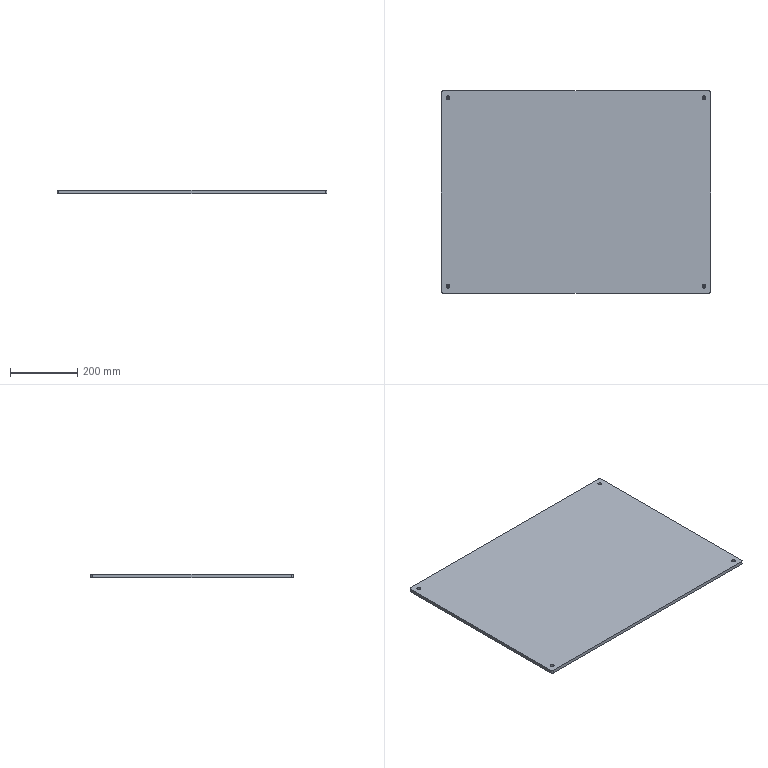Part | SolidWorks | features Extrusion 1, Fillet 1, HoleWzd 1 | 1 solid | 30 faces | box 800 x 600 x 10 mm | volume 4796860 mm3 | cylinder 20 | plane 10 | commonest cylinder face diameters 6.6 x8 11 x8 10 x4
STEP:
#1=CARTESIAN_POINT('',(-385.5,280.,3.6));
#2=VERTEX_POINT('',#1);
#3=CARTESIAN_POINT('',(-374.5,280.,3.6));
#4=VERTEX_POINT('',#3);
#5=CARTESIAN_POINT('',(-380.,280.,3.6));
#6=DIRECTION('',(0.,0.,1.));
#7=DIRECTION('',(1.,0.,0.));
#8=AXIS2_PLACEMENT_3D('',#5,#6,#7);
#9=CIRCLE('',#8,5.5);
#10=EDGE_CURVE('',#2,#4,#9,.T.);
#11=ORIENTED_EDGE('',*,*,#10,.F.);
#12=CARTESIAN_POINT('',(-385.5,280.,10.));
#13=VERTEX_POINT('',#12);
#14=CARTESIAN_POINT('',(-385.5,280.,10.));
#15=DIRECTION('',(0.,0.,1.));
#16=VECTOR('',#15,1000.);
#17=LINE('',#14,#16);
#18=EDGE_CURVE('',#2,#13,#17,.T.);
#19=ORIENTED_EDGE('',*,*,#18,.T.);
#20=CARTESIAN_POINT('',(-374.5,280.,10.));
#21=VERTEX_POINT('',#20);
#22=CARTESIAN_POINT('',(-380.,280.,10.));
#23=DIRECTION('',(0.,0.,1.));
#24=DIRECTION('',(1.,0.,0.));
#25=AXIS2_PLACEMENT_3D('',#22,#23,#24);
#26=CIRCLE('',#25,5.5);
#27=EDGE_CURVE('',#13,#21,#26,.T.);
#28=ORIENTED_EDGE('',*,*,#27,.T.);
#29=CARTESIAN_POINT('',(-374.5,280.,10.));
#30=DIRECTION('',(0.,0.,1.));
#31=VECTOR('',#30,1000.);
#32=LINE('',#29,#31);
#33=EDGE_CURVE('',#4,#21,#32,.T.);
#34=ORIENTED_EDGE('',*,*,#33,.F.);
#35=EDGE_LOOP('',(#11,#19,#28,#34));
#36=FACE_OUTER_BOUND('',#35,.T.);
#37=CARTESIAN_POINT('',(-380.,280.,10.));
#38=DIRECTION('',(0.,0.,1.));
#39=DIRECTION('',(1.,0.,0.));
#40=AXIS2_PLACEMENT_3D('',#37,#38,#39);
#41=CYLINDRICAL_SURFACE('',#40,5.5);
#42=ADVANCED_FACE('',(#36),#41,.F.);
#43=CARTESIAN_POINT('',(-383.3,280.,0.));
#44=VERTEX_POINT('',#43);
#45=CARTESIAN_POINT('',(-376.7,280.,0.));
#46=VERTEX_POINT('',#45);
#47=CARTESIAN_POINT('',(-380.,280.,0.));
#48=DIRECTION('',(0.,0.,1.));
#49=DIRECTION('',(1.,0.,0.));
#50=AXIS2_PLACEMENT_3D('',#47,#48,#49);
#51=CIRCLE('',#50,3.3);
#52=EDGE_CURVE('',#44,#46,#51,.T.);
#53=ORIENTED_EDGE('',*,*,#52,.F.);
#54=CARTESIAN_POINT('',(-383.3,280.,3.6));
#55=VERTEX_POINT('',#54);
#56=CARTESIAN_POINT('',(-383.3,280.,10.));
#57=DIRECTION('',(0.,0.,1.));
#58=VECTOR('',#57,1000.);
#59=LINE('',#56,#58);
#60=EDGE_CURVE('',#44,#55,#59,.T.);
#61=ORIENTED_EDGE('',*,*,#60,.T.);
#62=CARTESIAN_POINT('',(-376.7,280.,3.6));
#63=VERTEX_POINT('',#62);
#64=CARTESIAN_POINT('',(-380.,280.,3.6));
#65=DIRECTION('',(0.,0.,1.));
#66=DIRECTION('',(1.,0.,0.));
#67=AXIS2_PLACEMENT_3D('',#64,#65,#66);
#68=CIRCLE('',#67,3.3);
#69=EDGE_CURVE('',#55,#63,#68,.T.);
#70=ORIENTED_EDGE('',*,*,#69,.T.);
#71=CARTESIAN_POINT('',(-376.7,280.,10.));
#72=DIRECTION('',(0.,0.,1.));
#73=VECTOR('',#72,1000.);
#74=LINE('',#71,#73);
#75=EDGE_CURVE('',#46,#63,#74,.T.);
#76=ORIENTED_EDGE('',*,*,#75,.F.);
#77=EDGE_LOOP('',(#53,#61,#70,#76));
#78=FACE_OUTER_BOUND('',#77,.T.);
#79=CARTESIAN_POINT('',(-380.,280.,10.));
#80=DIRECTION('',(0.,0.,1.));
#81=DIRECTION('',(1.,0.,0.));
#82=AXIS2_PLACEMENT_3D('',#79,#80,#81);
#83=CYLINDRICAL_SURFACE('',#82,3.3);
#84=ADVANCED_FACE('',(#78),#83,.F.);
#85=CARTESIAN_POINT('',(374.5,280.,3.6));
#86=VERTEX_POINT('',#85);
#87=CARTESIAN_POINT('',(385.5,280.,3.6));
#88=VERTEX_POINT('',#87);
#89=CARTESIAN_POINT('',(380.,280.,3.6));
#90=DIRECTION('',(0.,0.,1.));
#91=DIRECTION('',(1.,0.,0.));
#92=AXIS2_PLACEMENT_3D('',#89,#90,#91);
#93=CIRCLE('',#92,5.5);
#94=EDGE_CURVE('',#86,#88,#93,.T.);
#95=ORIENTED_EDGE('',*,*,#94,.F.);
#96=CARTESIAN_POINT('',(374.5,280.,10.));
#97=VERTEX_POINT('',#96);
#98=CARTESIAN_POINT('',(374.5,280.,10.));
#99=DIRECTION('',(0.,0.,1.));
#100=VECTOR('',#99,1000.);
#101=LINE('',#98,#100);
#102=EDGE_CURVE('',#86,#97,#101,.T.);
#103=ORIENTED_EDGE('',*,*,#102,.T.);
#104=CARTESIAN_POINT('',(385.5,280.,10.));
#105=VERTEX_POINT('',#104);
#106=CARTESIAN_POINT('',(380.,280.,10.));
#107=DIRECTION('',(0.,0.,1.));
#108=DIRECTION('',(1.,0.,0.));
#109=AXIS2_PLACEMENT_3D('',#106,#107,#108);
#110=CIRCLE('',#109,5.5);
#111=EDGE_CURVE('',#97,#105,#110,.T.);
#112=ORIENTED_EDGE('',*,*,#111,.T.);
#113=CARTESIAN_POINT('',(385.5,280.,10.));
#114=DIRECTION('',(0.,0.,1.));
#115=VECTOR('',#114,1000.);
#116=LINE('',#113,#115);
#117=EDGE_CURVE('',#88,#105,#116,.T.);
#118=ORIENTED_EDGE('',*,*,#117,.F.);
#119=EDGE_LOOP('',(#95,#103,#112,#118));
#120=FACE_OUTER_BOUND('',#119,.T.);
#121=CARTESIAN_POINT('',(380.,280.,10.));
#122=DIRECTION('',(0.,0.,1.));
#123=DIRECTION('',(1.,0.,0.));
#124=AXIS2_PLACEMENT_3D('',#121,#122,#123);
#125=CYLINDRICAL_SURFACE('',#124,5.5);
#126=ADVANCED_FACE('',(#120),#125,.F.);
#127=CARTESIAN_POINT('',(376.7,280.,0.));
#128=VERTEX_POINT('',#127);
#129=CARTESIAN_POINT('',(383.3,280.,0.));
#130=VERTEX_POINT('',#129);
#131=CARTESIAN_POINT('',(380.,280.,0.));
#132=DIRECTION('',(0.,0.,1.));
#133=DIRECTION('',(1.,0.,0.));
#134=AXIS2_PLACEMENT_3D('',#131,#132,#133);
#135=CIRCLE('',#134,3.3);
#136=EDGE_CURVE('',#128,#130,#135,.T.);
#137=ORIENTED_EDGE('',*,*,#136,.F.);
#138=CARTESIAN_POINT('',(376.7,280.,3.6));
#139=VERTEX_POINT('',#138);
#140=CARTESIAN_POINT('',(376.7,280.,10.));
#141=DIRECTION('',(0.,0.,1.));
#142=VECTOR('',#141,1000.);
#143=LINE('',#140,#142);
#144=EDGE_CURVE('',#128,#139,#143,.T.);
#145=ORIENTED_EDGE('',*,*,#144,.T.);
#146=CARTESIAN_POINT('',(383.3,280.,3.6));
#147=VERTEX_POINT('',#146);
#148=CARTESIAN_POINT('',(380.,280.,3.6));
#149=DIRECTION('',(0.,0.,1.));
#150=DIRECTION('',(1.,0.,0.));
#151=AXIS2_PLACEMENT_3D('',#148,#149,#150);
#152=CIRCLE('',#151,3.3);
#153=EDGE_CURVE('',#139,#147,#152,.T.);
#154=ORIENTED_EDGE('',*,*,#153,.T.);
#155=CARTESIAN_POINT('',(383.3,280.,10.));
#156=DIRECTION('',(0.,0.,1.));
#157=VECTOR('',#156,1000.);
#158=LINE('',#155,#157);
#159=EDGE_CURVE('',#130,#147,#158,.T.);
#160=ORIENTED_EDGE('',*,*,#159,.F.);
#161=EDGE_LOOP('',(#137,#145,#154,#160));
#162=FACE_OUTER_BOUND('',#161,.T.);
#163=CARTESIAN_POINT('',(380.,280.,10.));
#164=DIRECTION('',(0.,0.,1.));
#165=DIRECTION('',(1.,0.,0.));
#166=AXIS2_PLACEMENT_3D('',#163,#164,#165);
#167=CYLINDRICAL_SURFACE('',#166,3.3);
#168=ADVANCED_FACE('',(#162),#167,.F.);
#169=CARTESIAN_POINT('',(374.5,-280.,3.6));
#170=VERTEX_POINT('',#169);
#171=CARTESIAN_POINT('',(385.5,-280.,3.6));
#172=VERTEX_POINT('',#171);
#173=CARTESIAN_POINT('',(380.,-280.,3.6));
#174=DIRECTION('',(0.,0.,1.));
#175=DIRECTION('',(1.,0.,0.));
#176=AXIS2_PLACEMENT_3D('',#173,#174,#175);
#177=CIRCLE('',#176,5.5);
#178=EDGE_CURVE('',#170,#172,#177,.T.);
#179=ORIENTED_EDGE('',*,*,#178,.F.);
#180=CARTESIAN_POINT('',(374.5,-280.,10.));
#181=VERTEX_POINT('',#180);
#182=CARTESIAN_POINT('',(374.5,-280.,10.));
#183=DIRECTION('',(0.,0.,1.));
#184=VECTOR('',#183,1000.);
#185=LINE('',#182,#184);
#186=EDGE_CURVE('',#170,#181,#185,.T.);
#187=ORIENTED_EDGE('',*,*,#186,.T.);
#188=CARTESIAN_POINT('',(385.5,-280.,10.));
#189=VERTEX_POINT('',#188);
#190=CARTESIAN_POINT('',(380.,-280.,10.));
#191=DIRECTION('',(0.,0.,1.));
#192=DIRECTION('',(1.,0.,0.));
#193=AXIS2_PLACEMENT_3D('',#190,#191,#192);
#194=CIRCLE('',#193,5.5);
#195=EDGE_CURVE('',#181,#189,#194,.T.);
#196=ORIENTED_EDGE('',*,*,#195,.T.);
#197=CARTESIAN_POINT('',(385.5,-280.,10.));
#198=DIRECTION('',(0.,0.,1.));
#199=VECTOR('',#198,1000.);
#200=LINE('',#197,#199);
#201=EDGE_CURVE('',#172,#189,#200,.T.);
#202=ORIENTED_EDGE('',*,*,#201,.F.);
#203=EDGE_LOOP('',(#179,#187,#196,#202));
#204=FACE_OUTER_BOUND('',#203,.T.);
#205=CARTESIAN_POINT('',(380.,-280.,10.));
#206=DIRECTION('',(0.,0.,1.));
#207=DIRECTION('',(1.,0.,0.));
#208=AXIS2_PLACEMENT_3D('',#205,#206,#207);
#209=CYLINDRICAL_SURFACE('',#208,5.5);
#210=ADVANCED_FACE('',(#204),#209,.F.);
#211=CARTESIAN_POINT('',(376.7,-280.,0.));
#212=VERTEX_POINT('',#211);
#213=CARTESIAN_POINT('',(383.3,-280.,0.));
#214=VERTEX_POINT('',#213);
#215=CARTESIAN_POINT('',(380.,-280.,0.));
#216=DIRECTION('',(0.,0.,1.));
#217=DIRECTION('',(1.,0.,0.));
#218=AXIS2_PLACEMENT_3D('',#215,#216,#217);
#219=CIRCLE('',#218,3.3);
#220=EDGE_CURVE('',#212,#214,#219,.T.);
#221=ORIENTED_EDGE('',*,*,#220,.F.);
#222=CARTESIAN_POINT('',(376.7,-280.,3.6));
#223=VERTEX_POINT('',#222);
#224=CARTESIAN_POINT('',(376.7,-280.,10.));
#225=DIRECTION('',(0.,0.,1.));
#226=VECTOR('',#225,1000.);
#227=LINE('',#224,#226);
#228=EDGE_CURVE('',#212,#223,#227,.T.);
#229=ORIENTED_EDGE('',*,*,#228,.T.);
#230=CARTESIAN_POINT('',(383.3,-280.,3.6));
#231=VERTEX_POINT('',#230);
#232=CARTESIAN_POINT('',(380.,-280.,3.6));
#233=DIRECTION('',(0.,0.,1.));
#234=DIRECTION('',(1.,0.,0.));
#235=AXIS2_PLACEMENT_3D('',#232,#233,#234);
#236=CIRCLE('',#235,3.3);
#237=EDGE_CURVE('',#223,#231,#236,.T.);
#238=ORIENTED_EDGE('',*,*,#237,.T.);
#239=CARTESIAN_POINT('',(383.3,-280.,10.));
#240=DIRECTION('',(0.,0.,1.));
#241=VECTOR('',#240,1000.);
#242=LINE('',#239,#241);
#243=EDGE_CURVE('',#214,#231,#242,.T.);
#244=ORIENTED_EDGE('',*,*,#243,.F.);
#245=EDGE_LOOP('',(#221,#229,#238,#244));
#246=FACE_OUTER_BOUND('',#245,.T.);
#247=CARTESIAN_POINT('',(380.,-280.,10.));
#248=DIRECTION('',(0.,0.,1.));
#249=DIRECTION('',(1.,0.,0.));
#250=AXIS2_PLACEMENT_3D('',#247,#248,#249);
#251=CYLINDRICAL_SURFACE('',#250,3.3);
#252=ADVANCED_FACE('',(#246),#251,.F.);
#253=CARTESIAN_POINT('',(-385.5,-280.,3.6));
#254=VERTEX_POINT('',#253);
#255=CARTESIAN_POINT('',(-374.5,-280.,3.6));
#256=VERTEX_POINT('',#255);
#257=CARTESIAN_POINT('',(-380.,-280.,3.6));
#258=DIRECTION('',(0.,0.,1.));
#259=DIRECTION('',(1.,0.,0.));
#260=AXIS2_PLACEMENT_3D('',#257,#258,#259);
#261=CIRCLE('',#260,5.5);
#262=EDGE_CURVE('',#254,#256,#261,.T.);
#263=ORIENTED_EDGE('',*,*,#262,.F.);
#264=CARTESIAN_POINT('',(-385.5,-280.,10.));
#265=VERTEX_POINT('',#264);
#266=CARTESIAN_POINT('',(-385.5,-280.,10.));
#267=DIRECTION('',(0.,0.,1.));
#268=VECTOR('',#267,1000.);
#269=LINE('',#266,#268);
#270=EDGE_CURVE('',#254,#265,#269,.T.);
#271=ORIENTED_EDGE('',*,*,#270,.T.);
#272=CARTESIAN_POINT('',(-374.5,-280.,10.));
#273=VERTEX_POINT('',#272);
#274=CARTESIAN_POINT('',(-380.,-280.,10.));
#275=DIRECTION('',(0.,0.,1.));
#276=DIRECTION('',(1.,0.,0.));
#277=AXIS2_PLACEMENT_3D('',#274,#275,#276);
#278=CIRCLE('',#277,5.5);
#279=EDGE_CURVE('',#265,#273,#278,.T.);
#280=ORIENTED_EDGE('',*,*,#279,.T.);
#281=CARTESIAN_POINT('',(-374.5,-280.,10.));
#282=DIRECTION('',(0.,0.,1.));
#283=VECTOR('',#282,1000.);
#284=LINE('',#281,#283);
#285=EDGE_CURVE('',#256,#273,#284,.T.);
#286=ORIENTED_EDGE('',*,*,#285,.F.);
#287=EDGE_LOOP('',(#263,#271,#280,#286));
#288=FACE_OUTER_BOUND('',#287,.T.);
#289=CARTESIAN_POINT('',(-380.,-280.,10.));
#290=DIRECTION('',(0.,0.,1.));
#291=DIRECTION('',(1.,0.,0.));
#292=AXIS2_PLACEMENT_3D('',#289,#290,#291);
#293=CYLINDRICAL_SURFACE('',#292,5.5);
#294=ADVANCED_FACE('',(#288),#293,.F.);
#295=CARTESIAN_POINT('',(-383.3,-280.,0.));
#296=VERTEX_POINT('',#295);
#297=CARTESIAN_POINT('',(-376.7,-280.,0.));
#298=VERTEX_POINT('',#297);
#299=CARTESIAN_POINT('',(-380.,-280.,0.));
#300=DIRECTION('',(0.,0.,1.));
#301=DIRECTION('',(1.,0.,0.));
#302=AXIS2_PLACEMENT_3D('',#299,#300,#301);
#303=CIRCLE('',#302,3.3);
#304=EDGE_CURVE('',#296,#298,#303,.T.);
#305=ORIENTED_EDGE('',*,*,#304,.F.);
#306=CARTESIAN_POINT('',(-383.3,-280.,3.6));
#307=VERTEX_POINT('',#306);
#308=CARTESIAN_POINT('',(-383.3,-280.,10.));
#309=DIRECTION('',(0.,0.,1.));
#310=VECTOR('',#309,1000.);
#311=LINE('',#308,#310);
#312=EDGE_CURVE('',#296,#307,#311,.T.);
#313=ORIENTED_EDGE('',*,*,#312,.T.);
#314=CARTESIAN_POINT('',(-376.7,-280.,3.6));
#315=VERTEX_POINT('',#314);
#316=CARTESIAN_POINT('',(-380.,-280.,3.6));
#317=DIRECTION('',(0.,0.,1.));
#318=DIRECTION('',(1.,0.,0.));
#319=AXIS2_PLACEMENT_3D('',#316,#317,#318);
#320=CIRCLE('',#319,3.3);
#321=EDGE_CURVE('',#307,#315,#320,.T.);
#322=ORIENTED_EDGE('',*,*,#321,.T.);
#323=CARTESIAN_POINT('',(-376.7,-280.,10.));
#324=DIRECTION('',(0.,0.,1.));
#325=VECTOR('',#324,1000.);
#326=LINE('',#323,#325);
#327=EDGE_CURVE('',#298,#315,#326,.T.);
#328=ORIENTED_EDGE('',*,*,#327,.F.);
#329=EDGE_LOOP('',(#305,#313,#322,#328));
#330=FACE_OUTER_BOUND('',#329,.T.);
#331=CARTESIAN_POINT('',(-380.,-280.,10.));
#332=DIRECTION('',(0.,0.,1.));
#333=DIRECTION('',(1.,0.,0.));
#334=AXIS2_PLACEMENT_3D('',#331,#332,#333);
#335=CYLINDRICAL_SURFACE('',#334,3.3);
#336=ADVANCED_FACE('',(#330),#335,.F.);
#337=CARTESIAN_POINT('',(400.,-295.,0.));
#338=VERTEX_POINT('',#337);
#339=CARTESIAN_POINT('',(400.,295.,0.));
#340=VERTEX_POINT('',#339);
#341=CARTESIAN_POINT('',(400.,300.,0.));
#342=DIRECTION('',(0.,1.,0.));
#343=VECTOR('',#342,1000.);
#344=LINE('',#341,#343);
#345=EDGE_CURVE('',#338,#340,#344,.T.);
#346=ORIENTED_EDGE('',*,*,#345,.T.);
#347=CARTESIAN_POINT('',(400.,295.,10.));
#348=VERTEX_POINT('',#347);
#349=CARTESIAN_POINT('',(400.,295.,10.));
#350=DIRECTION('',(0.,0.,1.));
#351=VECTOR('',#350,1000.);
#352=LINE('',#349,#351);
#353=EDGE_CURVE('',#340,#348,#352,.T.);
#354=ORIENTED_EDGE('',*,*,#353,.T.);
#355=CARTESIAN_POINT('',(400.,-295.,10.));
#356=VERTEX_POINT('',#355);
#357=CARTESIAN_POINT('',(400.,300.,10.));
#358=DIRECTION('',(0.,1.,0.));
#359=VECTOR('',#358,1000.);
#360=LINE('',#357,#359);
#361=EDGE_CURVE('',#356,#348,#360,.T.);
#362=ORIENTED_EDGE('',*,*,#361,.F.);
#363=CARTESIAN_POINT('',(400.,-295.,10.));
#364=DIRECTION('',(0.,0.,-1.));
#365=VECTOR('',#364,1000.);
#366=LINE('',#363,#365);
#367=EDGE_CURVE('',#356,#338,#366,.T.);
#368=ORIENTED_EDGE('',*,*,#367,.T.);
#369=EDGE_LOOP('',(#346,#354,#362,#368));
#370=FACE_OUTER_BOUND('',#369,.T.);
#371=CARTESIAN_POINT('',(400.,300.,10.));
#372=DIRECTION('',(-1.,0.,0.));
#373=DIRECTION('',(0.,0.,1.));
#374=AXIS2_PLACEMENT_3D('',#371,#372,#373);
#375=PLANE('',#374);
#376=ADVANCED_FACE('',(#370),#375,.F.);
#377=CARTESIAN_POINT('',(395.,300.,10.));
#378=VERTEX_POINT('',#377);
#379=CARTESIAN_POINT('',(-395.,300.,10.));
#380=VERTEX_POINT('',#379);
#381=CARTESIAN_POINT('',(-400.,300.,10.));
#382=DIRECTION('',(-1.,0.,0.));
#383=VECTOR('',#382,1000.);
#384=LINE('',#381,#383);
#385=EDGE_CURVE('',#378,#380,#384,.T.);
#386=ORIENTED_EDGE('',*,*,#385,.F.);
#387=CARTESIAN_POINT('',(395.,300.,0.));
#388=VERTEX_POINT('',#387);
#389=CARTESIAN_POINT('',(395.,300.,10.));
#390=DIRECTION('',(0.,0.,-1.));
#391=VECTOR('',#390,1000.);
#392=LINE('',#389,#391);
#393=EDGE_CURVE('',#378,#388,#392,.T.);
#394=ORIENTED_EDGE('',*,*,#393,.T.);
#395=CARTESIAN_POINT('',(-395.,300.,0.));
#396=VERTEX_POINT('',#395);
#397=CARTESIAN_POINT('',(-400.,300.,0.));
#398=DIRECTION('',(-1.,0.,0.));
#399=VECTOR('',#398,1000.);
#400=LINE('',#397,#399);
#401=EDGE_CURVE('',#388,#396,#400,.T.);
#402=ORIENTED_EDGE('',*,*,#401,.T.);
#403=CARTESIAN_POINT('',(-395.,300.,10.));
#404=DIRECTION('',(0.,0.,1.));
#405=VECTOR('',#404,1000.);
#406=LINE('',#403,#405);
#407=EDGE_CURVE('',#396,#380,#406,.T.);
#408=ORIENTED_EDGE('',*,*,#407,.T.);
#409=EDGE_LOOP('',(#386,#394,#402,#408));
#410=FACE_OUTER_BOUND('',#409,.T.);
#411=CARTESIAN_POINT('',(-400.,300.,10.));
#412=DIRECTION('',(0.,-1.,0.));
#413=DIRECTION('',(0.,0.,-1.));
#414=AXIS2_PLACEMENT_3D('',#411,#412,#413);
#415=PLANE('',#414);
#416=ADVANCED_FACE('',(#410),#415,.F.);
#417=CARTESIAN_POINT('',(-400.,295.,0.));
#418=VERTEX_POINT('',#417);
#419=CARTESIAN_POINT('',(-400.,-295.,0.));
#420=VERTEX_POINT('',#419);
#421=CARTESIAN_POINT('',(-400.,300.,0.));
#422=DIRECTION('',(0.,-1.,0.));
#423=VECTOR('',#422,1000.);
#424=LINE('',#421,#423);
#425=EDGE_CURVE('',#418,#420,#424,.T.);
#426=ORIENTED_EDGE('',*,*,#425,.T.);
#427=CARTESIAN_POINT('',(-400.,-295.,10.));
#428=VERTEX_POINT('',#427);
#429=CARTESIAN_POINT('',(-400.,-295.,10.));
#430=DIRECTION('',(0.,0.,1.));
#431=VECTOR('',#430,1000.);
#432=LINE('',#429,#431);
#433=EDGE_CURVE('',#420,#428,#432,.T.);
#434=ORIENTED_EDGE('',*,*,#433,.T.);
#435=CARTESIAN_POINT('',(-400.,295.,10.));
#436=VERTEX_POINT('',#435);
#437=CARTESIAN_POINT('',(-400.,300.,10.));
#438=DIRECTION('',(0.,-1.,0.));
#439=VECTOR('',#438,1000.);
#440=LINE('',#437,#439);
#441=EDGE_CURVE('',#436,#428,#440,.T.);
#442=ORIENTED_EDGE('',*,*,#441,.F.);
#443=CARTESIAN_POINT('',(-400.,295.,10.));
#444=DIRECTION('',(0.,0.,-1.));
#445=VECTOR('',#444,1000.);
#446=LINE('',#443,#445);
#447=EDGE_CURVE('',#436,#418,#446,.T.);
#448=ORIENTED_EDGE('',*,*,#447,.T.);
#449=EDGE_LOOP('',(#426,#434,#442,#448));
#450=FACE_OUTER_BOUND('',#449,.T.);
#451=CARTESIAN_POINT('',(-400.,300.,10.));
#452=DIRECTION('',(1.,0.,0.));
#453=DIRECTION('',(0.,0.,-1.));
#454=AXIS2_PLACEMENT_3D('',#451,#452,#453);
#455=PLANE('',#454);
#456=ADVANCED_FACE('',(#450),#455,.F.);
#457=CARTESIAN_POINT('',(-395.,-300.,0.));
#458=VERTEX_POINT('',#457);
#459=CARTESIAN_POINT('',(395.,-300.,0.));
#460=VERTEX_POINT('',#459);
#461=CARTESIAN_POINT('',(-400.,-300.,0.));
#462=DIRECTION('',(1.,0.,0.));
#463=VECTOR('',#462,1000.);
#464=LINE('',#461,#463);
#465=EDGE_CURVE('',#458,#460,#464,.T.);
#466=ORIENTED_EDGE('',*,*,#465,.T.);
#467=CARTESIAN_POINT('',(395.,-300.,10.));
#468=VERTEX_POINT('',#467);
#469=CARTESIAN_POINT('',(395.,-300.,10.));
#470=DIRECTION('',(0.,0.,1.));
#471=VECTOR('',#470,1000.);
#472=LINE('',#469,#471);
#473=EDGE_CURVE('',#460,#468,#472,.T.);
#474=ORIENTED_EDGE('',*,*,#473,.T.);
#475=CARTESIAN_POINT('',(-395.,-300.,10.));
#476=VERTEX_POINT('',#475);
#477=CARTESIAN_POINT('',(-400.,-300.,10.));
#478=DIRECTION('',(1.,0.,0.));
#479=VECTOR('',#478,1000.);
#480=LINE('',#477,#479);
#481=EDGE_CURVE('',#476,#468,#480,.T.);
#482=ORIENTED_EDGE('',*,*,#481,.F.);
#483=CARTESIAN_POINT('',(-395.,-300.,10.));
#484=DIRECTION('',(0.,0.,-1.));
#485=VECTOR('',#484,1000.);
#486=LINE('',#483,#485);
#487=EDGE_CURVE('',#476,#458,#486,.T.);
#488=ORIENTED_EDGE('',*,*,#487,.T.);
#489=EDGE_LOOP('',(#466,#474,#482,#488));
#490=FACE_OUTER_BOUND('',#489,.T.);
#491=CARTESIAN_POINT('',(-400.,-300.,10.));
#492=DIRECTION('',(0.,1.,0.));
#493=DIRECTION('',(0.,0.,1.));
#494=AXIS2_PLACEMENT_3D('',#491,#492,#493);
#495=PLANE('',#494);
#496=ADVANCED_FACE('',(#490),#495,.F.);
#497=CARTESIAN_POINT('',(-380.,280.,10.));
#498=DIRECTION('',(0.,0.,1.));
#499=DIRECTION('',(1.,0.,0.));
#500=AXIS2_PLACEMENT_3D('',#497,#498,#499);
#501=CIRCLE('',#500,5.5);
#502=EDGE_CURVE('',#21,#13,#501,.T.);
#503=ORIENTED_EDGE('',*,*,#502,.F.);
#504=ORIENTED_EDGE('',*,*,#27,.F.);
#505=EDGE_LOOP('',(#503,#504));
#506=FACE_BOUND('',#505,.T.);
#507=CARTESIAN_POINT('',(380.,280.,10.));
#508=DIRECTION('',(0.,0.,1.));
#509=DIRECTION('',(1.,0.,0.));
#510=AXIS2_PLACEMENT_3D('',#507,#508,#509);
#511=CIRCLE('',#510,5.5);
#512=EDGE_CURVE('',#105,#97,#511,.T.);
#513=ORIENTED_EDGE('',*,*,#512,.F.);
#514=ORIENTED_EDGE('',*,*,#111,.F.);
#515=EDGE_LOOP('',(#513,#514));
#516=FACE_BOUND('',#515,.T.);
#517=CARTESIAN_POINT('',(380.,-280.,10.));
#518=DIRECTION('',(0.,0.,1.));
#519=DIRECTION('',(1.,0.,0.));
#520=AXIS2_PLACEMENT_3D('',#517,#518,#519);
#521=CIRCLE('',#520,5.5);
#522=EDGE_CURVE('',#189,#181,#521,.T.);
#523=ORIENTED_EDGE('',*,*,#522,.F.);
#524=ORIENTED_EDGE('',*,*,#195,.F.);
#525=EDGE_LOOP('',(#523,#524));
#526=FACE_BOUND('',#525,.T.);
#527=CARTESIAN_POINT('',(-380.,-280.,10.));
#528=DIRECTION('',(0.,0.,1.));
#529=DIRECTION('',(1.,0.,0.));
#530=AXIS2_PLACEMENT_3D('',#527,#528,#529);
#531=CIRCLE('',#530,5.5);
#532=EDGE_CURVE('',#273,#265,#531,.T.);
#533=ORIENTED_EDGE('',*,*,#532,.F.);
#534=ORIENTED_EDGE('',*,*,#279,.F.);
#535=EDGE_LOOP('',(#533,#534));
#536=FACE_BOUND('',#535,.T.);
#537=ORIENTED_EDGE('',*,*,#361,.T.);
#538=CARTESIAN_POINT('',(395.,295.,10.));
#539=DIRECTION('',(0.,0.,1.));
#540=DIRECTION('',(1.,0.,0.));
#541=AXIS2_PLACEMENT_3D('',#538,#539,#540);
#542=CIRCLE('',#541,5.);
#543=EDGE_CURVE('',#348,#378,#542,.T.);
#544=ORIENTED_EDGE('',*,*,#543,.T.);
#545=ORIENTED_EDGE('',*,*,#385,.T.);
#546=CARTESIAN_POINT('',(-395.,295.,10.));
#547=DIRECTION('',(0.,0.,1.));
#548=DIRECTION('',(1.,0.,0.));
#549=AXIS2_PLACEMENT_3D('',#546,#547,#548);
#550=CIRCLE('',#549,5.);
#551=EDGE_CURVE('',#380,#436,#550,.T.);
#552=ORIENTED_EDGE('',*,*,#551,.T.);
#553=ORIENTED_EDGE('',*,*,#441,.T.);
#554=CARTESIAN_POINT('',(-395.,-295.,10.));
#555=DIRECTION('',(0.,0.,1.));
#556=DIRECTION('',(1.,0.,0.));
#557=AXIS2_PLACEMENT_3D('',#554,#555,#556);
#558=CIRCLE('',#557,5.);
#559=EDGE_CURVE('',#428,#476,#558,.T.);
#560=ORIENTED_EDGE('',*,*,#559,.T.);
#561=ORIENTED_EDGE('',*,*,#481,.T.);
#562=CARTESIAN_POINT('',(395.,-295.,10.));
#563=DIRECTION('',(0.,0.,1.));
#564=DIRECTION('',(1.,0.,0.));
#565=AXIS2_PLACEMENT_3D('',#562,#563,#564);
#566=CIRCLE('',#565,5.);
#567=EDGE_CURVE('',#468,#356,#566,.T.);
#568=ORIENTED_EDGE('',*,*,#567,.T.);
#569=EDGE_LOOP('',(#537,#544,#545,#552,#553,#560,#561,#568));
#570=FACE_OUTER_BOUND('',#569,.T.);
#571=CARTESIAN_POINT('',(0.,0.,10.));
#572=DIRECTION('',(0.,0.,1.));
#573=DIRECTION('',(1.,0.,0.));
#574=AXIS2_PLACEMENT_3D('',#571,#572,#573);
#575=PLANE('',#574);
#576=ADVANCED_FACE('',(#506,#516,#526,#536,#570),#575,.T.);
#577=CARTESIAN_POINT('',(-380.,280.,0.));
#578=DIRECTION('',(0.,0.,1.));
#579=DIRECTION('',(1.,0.,0.));
#580=AXIS2_PLACEMENT_3D('',#577,#578,#579);
#581=CIRCLE('',#580,3.3);
#582=EDGE_CURVE('',#46,#44,#581,.T.);
#583=ORIENTED_EDGE('',*,*,#582,.T.);
#584=ORIENTED_EDGE('',*,*,#52,.T.);
#585=EDGE_LOOP('',(#583,#584));
#586=FACE_BOUND('',#585,.T.);
#587=CARTESIAN_POINT('',(380.,280.,0.));
#588=DIRECTION('',(0.,0.,1.));
#589=DIRECTION('',(1.,0.,0.));
#590=AXIS2_PLACEMENT_3D('',#587,#588,#589);
#591=CIRCLE('',#590,3.3);
#592=EDGE_CURVE('',#130,#128,#591,.T.);
#593=ORIENTED_EDGE('',*,*,#592,.T.);
#594=ORIENTED_EDGE('',*,*,#136,.T.);
#595=EDGE_LOOP('',(#593,#594));
#596=FACE_BOUND('',#595,.T.);
#597=CARTESIAN_POINT('',(380.,-280.,0.));
#598=DIRECTION('',(0.,0.,1.));
#599=DIRECTION('',(1.,0.,0.));
#600=AXIS2_PLACEMENT_3D('',#597,#598,#599);
#601=CIRCLE('',#600,3.3);
#602=EDGE_CURVE('',#214,#212,#601,.T.);
#603=ORIENTED_EDGE('',*,*,#602,.T.);
#604=ORIENTED_EDGE('',*,*,#220,.T.);
#605=EDGE_LOOP('',(#603,#604));
#606=FACE_BOUND('',#605,.T.);
#607=CARTESIAN_POINT('',(-380.,-280.,0.));
#608=DIRECTION('',(0.,0.,1.));
#609=DIRECTION('',(1.,0.,0.));
#610=AXIS2_PLACEMENT_3D('',#607,#608,#609);
#611=CIRCLE('',#610,3.3);
#612=EDGE_CURVE('',#298,#296,#611,.T.);
#613=ORIENTED_EDGE('',*,*,#612,.T.);
#614=ORIENTED_EDGE('',*,*,#304,.T.);
#615=EDGE_LOOP('',(#613,#614));
#616=FACE_BOUND('',#615,.T.);
#617=ORIENTED_EDGE('',*,*,#401,.F.);
#618=CARTESIAN_POINT('',(395.,295.,0.));
#619=DIRECTION('',(0.,0.,-1.));
#620=DIRECTION('',(1.,0.,0.));
#621=AXIS2_PLACEMENT_3D('',#618,#619,#620);
#622=CIRCLE('',#621,5.);
#623=EDGE_CURVE('',#388,#340,#622,.T.);
#624=ORIENTED_EDGE('',*,*,#623,.T.);
#625=ORIENTED_EDGE('',*,*,#345,.F.);
#626=CARTESIAN_POINT('',(395.,-295.,0.));
#627=DIRECTION('',(0.,0.,-1.));
#628=DIRECTION('',(1.,0.,0.));
#629=AXIS2_PLACEMENT_3D('',#626,#627,#628);
#630=CIRCLE('',#629,5.);
#631=EDGE_CURVE('',#338,#460,#630,.T.);
#632=ORIENTED_EDGE('',*,*,#631,.T.);
#633=ORIENTED_EDGE('',*,*,#465,.F.);
#634=CARTESIAN_POINT('',(-395.,-295.,0.));
#635=DIRECTION('',(0.,0.,-1.));
#636=DIRECTION('',(1.,0.,0.));
#637=AXIS2_PLACEMENT_3D('',#634,#635,#636);
#638=CIRCLE('',#637,5.);
#639=EDGE_CURVE('',#458,#420,#638,.T.);
#640=ORIENTED_EDGE('',*,*,#639,.T.);
#641=ORIENTED_EDGE('',*,*,#425,.F.);
#642=CARTESIAN_POINT('',(-395.,295.,0.));
#643=DIRECTION('',(0.,0.,-1.));
#644=DIRECTION('',(1.,0.,0.));
#645=AXIS2_PLACEMENT_3D('',#642,#643,#644);
#646=CIRCLE('',#645,5.);
#647=EDGE_CURVE('',#418,#396,#646,.T.);
#648=ORIENTED_EDGE('',*,*,#647,.T.);
#649=EDGE_LOOP('',(#617,#624,#625,#632,#633,#640,#641,#648));
#650=FACE_OUTER_BOUND('',#649,.T.);
#651=CARTESIAN_POINT('',(0.,0.,0.));
#652=DIRECTION('',(0.,0.,1.));
#653=DIRECTION('',(1.,0.,0.));
#654=AXIS2_PLACEMENT_3D('',#651,#652,#653);
#655=PLANE('',#654);
#656=ADVANCED_FACE('',(#586,#596,#606,#616,#650),#655,.F.);
#657=ORIENTED_EDGE('',*,*,#312,.F.);
#658=ORIENTED_EDGE('',*,*,#612,.F.);
#659=ORIENTED_EDGE('',*,*,#327,.T.);
#660=CARTESIAN_POINT('',(-380.,-280.,3.6));
#661=DIRECTION('',(0.,0.,1.));
#662=DIRECTION('',(1.,0.,0.));
#663=AXIS2_PLACEMENT_3D('',#660,#661,#662);
#664=CIRCLE('',#663,3.3);
#665=EDGE_CURVE('',#315,#307,#664,.T.);
#666=ORIENTED_EDGE('',*,*,#665,.T.);
#667=EDGE_LOOP('',(#657,#658,#659,#666));
#668=FACE_OUTER_BOUND('',#667,.T.);
#669=CARTESIAN_POINT('',(-380.,-280.,10.));
#670=DIRECTION('',(0.,0.,1.));
#671=DIRECTION('',(1.,0.,0.));
#672=AXIS2_PLACEMENT_3D('',#669,#670,#671);
#673=CYLINDRICAL_SURFACE('',#672,3.3);
#674=ADVANCED_FACE('',(#668),#673,.F.);
#675=ORIENTED_EDGE('',*,*,#665,.F.);
#676=ORIENTED_EDGE('',*,*,#321,.F.);
#677=EDGE_LOOP('',(#675,#676));
#678=FACE_BOUND('',#677,.T.);
#679=CARTESIAN_POINT('',(-380.,-280.,3.6));
#680=DIRECTION('',(0.,0.,1.));
#681=DIRECTION('',(1.,0.,0.));
#682=AXIS2_PLACEMENT_3D('',#679,#680,#681);
#683=CIRCLE('',#682,5.5);
#684=EDGE_CURVE('',#256,#254,#683,.T.);
#685=ORIENTED_EDGE('',*,*,#684,.T.);
#686=ORIENTED_EDGE('',*,*,#262,.T.);
#687=EDGE_LOOP('',(#685,#686));
#688=FACE_OUTER_BOUND('',#687,.T.);
#689=CARTESIAN_POINT('',(-376.7,-280.,3.6));
#690=DIRECTION('',(0.,0.,-1.));
#691=DIRECTION('',(-1.,0.,0.));
#692=AXIS2_PLACEMENT_3D('',#689,#690,#691);
#693=PLANE('',#692);
#694=ADVANCED_FACE('',(#678,#688),#693,.F.);
#695=ORIENTED_EDGE('',*,*,#270,.F.);
#696=ORIENTED_EDGE('',*,*,#684,.F.);
#697=ORIENTED_EDGE('',*,*,#285,.T.);
#698=ORIENTED_EDGE('',*,*,#532,.T.);
#699=EDGE_LOOP('',(#695,#696,#697,#698));
#700=FACE_OUTER_BOUND('',#699,.T.);
#701=CARTESIAN_POINT('',(-380.,-280.,10.));
#702=DIRECTION('',(0.,0.,1.));
#703=DIRECTION('',(1.,0.,0.));
#704=AXIS2_PLACEMENT_3D('',#701,#702,#703);
#705=CYLINDRICAL_SURFACE('',#704,5.5);
#706=ADVANCED_FACE('',(#700),#705,.F.);
#707=ORIENTED_EDGE('',*,*,#228,.F.);
#708=ORIENTED_EDGE('',*,*,#602,.F.);
#709=ORIENTED_EDGE('',*,*,#243,.T.);
#710=CARTESIAN_POINT('',(380.,-280.,3.6));
#711=DIRECTION('',(0.,0.,1.));
#712=DIRECTION('',(1.,0.,0.));
#713=AXIS2_PLACEMENT_3D('',#710,#711,#712);
#714=CIRCLE('',#713,3.3);
#715=EDGE_CURVE('',#231,#223,#714,.T.);
#716=ORIENTED_EDGE('',*,*,#715,.T.);
#717=EDGE_LOOP('',(#707,#708,#709,#716));
#718=FACE_OUTER_BOUND('',#717,.T.);
#719=CARTESIAN_POINT('',(380.,-280.,10.));
#720=DIRECTION('',(0.,0.,1.));
#721=DIRECTION('',(1.,0.,0.));
#722=AXIS2_PLACEMENT_3D('',#719,#720,#721);
#723=CYLINDRICAL_SURFACE('',#722,3.3);
#724=ADVANCED_FACE('',(#718),#723,.F.);
#725=ORIENTED_EDGE('',*,*,#715,.F.);
#726=ORIENTED_EDGE('',*,*,#237,.F.);
#727=EDGE_LOOP('',(#725,#726));
#728=FACE_BOUND('',#727,.T.);
#729=CARTESIAN_POINT('',(380.,-280.,3.6));
#730=DIRECTION('',(0.,0.,1.));
#731=DIRECTION('',(1.,0.,0.));
#732=AXIS2_PLACEMENT_3D('',#729,#730,#731);
#733=CIRCLE('',#732,5.5);
#734=EDGE_CURVE('',#172,#170,#733,.T.);
#735=ORIENTED_EDGE('',*,*,#734,.T.);
#736=ORIENTED_EDGE('',*,*,#178,.T.);
#737=EDGE_LOOP('',(#735,#736));
#738=FACE_OUTER_BOUND('',#737,.T.);
#739=CARTESIAN_POINT('',(383.3,-280.,3.6));
#740=DIRECTION('',(0.,0.,-1.));
#741=DIRECTION('',(-1.,0.,0.));
#742=AXIS2_PLACEMENT_3D('',#739,#740,#741);
#743=PLANE('',#742);
#744=ADVANCED_FACE('',(#728,#738),#743,.F.);
#745=ORIENTED_EDGE('',*,*,#186,.F.);
#746=ORIENTED_EDGE('',*,*,#734,.F.);
#747=ORIENTED_EDGE('',*,*,#201,.T.);
#748=ORIENTED_EDGE('',*,*,#522,.T.);
#749=EDGE_LOOP('',(#745,#746,#747,#748));
#750=FACE_OUTER_BOUND('',#749,.T.);
#751=CARTESIAN_POINT('',(380.,-280.,10.));
#752=DIRECTION('',(0.,0.,1.));
#753=DIRECTION('',(1.,0.,0.));
#754=AXIS2_PLACEMENT_3D('',#751,#752,#753);
#755=CYLINDRICAL_SURFACE('',#754,5.5);
#756=ADVANCED_FACE('',(#750),#755,.F.);
#757=ORIENTED_EDGE('',*,*,#144,.F.);
#758=ORIENTED_EDGE('',*,*,#592,.F.);
#759=ORIENTED_EDGE('',*,*,#159,.T.);
#760=CARTESIAN_POINT('',(380.,280.,3.6));
#761=DIRECTION('',(0.,0.,1.));
#762=DIRECTION('',(1.,0.,0.));
#763=AXIS2_PLACEMENT_3D('',#760,#761,#762);
#764=CIRCLE('',#763,3.3);
#765=EDGE_CURVE('',#147,#139,#764,.T.);
#766=ORIENTED_EDGE('',*,*,#765,.T.);
#767=EDGE_LOOP('',(#757,#758,#759,#766));
#768=FACE_OUTER_BOUND('',#767,.T.);
#769=CARTESIAN_POINT('',(380.,280.,10.));
#770=DIRECTION('',(0.,0.,1.));
#771=DIRECTION('',(1.,0.,0.));
#772=AXIS2_PLACEMENT_3D('',#769,#770,#771);
#773=CYLINDRICAL_SURFACE('',#772,3.3);
#774=ADVANCED_FACE('',(#768),#773,.F.);
#775=ORIENTED_EDGE('',*,*,#765,.F.);
#776=ORIENTED_EDGE('',*,*,#153,.F.);
#777=EDGE_LOOP('',(#775,#776));
#778=FACE_BOUND('',#777,.T.);
#779=CARTESIAN_POINT('',(380.,280.,3.6));
#780=DIRECTION('',(0.,0.,1.));
#781=DIRECTION('',(1.,0.,0.));
#782=AXIS2_PLACEMENT_3D('',#779,#780,#781);
#783=CIRCLE('',#782,5.5);
#784=EDGE_CURVE('',#88,#86,#783,.T.);
#785=ORIENTED_EDGE('',*,*,#784,.T.);
#786=ORIENTED_EDGE('',*,*,#94,.T.);
#787=EDGE_LOOP('',(#785,#786));
#788=FACE_OUTER_BOUND('',#787,.T.);
#789=CARTESIAN_POINT('',(383.3,280.,3.6));
#790=DIRECTION('',(0.,0.,-1.));
#791=DIRECTION('',(-1.,0.,0.));
#792=AXIS2_PLACEMENT_3D('',#789,#790,#791);
#793=PLANE('',#792);
#794=ADVANCED_FACE('',(#778,#788),#793,.F.);
#795=ORIENTED_EDGE('',*,*,#102,.F.);
#796=ORIENTED_EDGE('',*,*,#784,.F.);
#797=ORIENTED_EDGE('',*,*,#117,.T.);
#798=ORIENTED_EDGE('',*,*,#512,.T.);
#799=EDGE_LOOP('',(#795,#796,#797,#798));
#800=FACE_OUTER_BOUND('',#799,.T.);
#801=CARTESIAN_POINT('',(380.,280.,10.));
#802=DIRECTION('',(0.,0.,1.));
#803=DIRECTION('',(1.,0.,0.));
#804=AXIS2_PLACEMENT_3D('',#801,#802,#803);
#805=CYLINDRICAL_SURFACE('',#804,5.5);
#806=ADVANCED_FACE('',(#800),#805,.F.);
#807=ORIENTED_EDGE('',*,*,#60,.F.);
#808=ORIENTED_EDGE('',*,*,#582,.F.);
#809=ORIENTED_EDGE('',*,*,#75,.T.);
#810=CARTESIAN_POINT('',(-380.,280.,3.6));
#811=DIRECTION('',(0.,0.,1.));
#812=DIRECTION('',(1.,0.,0.));
#813=AXIS2_PLACEMENT_3D('',#810,#811,#812);
#814=CIRCLE('',#813,3.3);
#815=EDGE_CURVE('',#63,#55,#814,.T.);
#816=ORIENTED_EDGE('',*,*,#815,.T.);
#817=EDGE_LOOP('',(#807,#808,#809,#816));
#818=FACE_OUTER_BOUND('',#817,.T.);
#819=CARTESIAN_POINT('',(-380.,280.,10.));
#820=DIRECTION('',(0.,0.,1.));
#821=DIRECTION('',(1.,0.,0.));
#822=AXIS2_PLACEMENT_3D('',#819,#820,#821);
#823=CYLINDRICAL_SURFACE('',#822,3.3);
#824=ADVANCED_FACE('',(#818),#823,.F.);
#825=ORIENTED_EDGE('',*,*,#815,.F.);
#826=ORIENTED_EDGE('',*,*,#69,.F.);
#827=EDGE_LOOP('',(#825,#826));
#828=FACE_BOUND('',#827,.T.);
#829=CARTESIAN_POINT('',(-380.,280.,3.6));
#830=DIRECTION('',(0.,0.,1.));
#831=DIRECTION('',(1.,0.,0.));
#832=AXIS2_PLACEMENT_3D('',#829,#830,#831);
#833=CIRCLE('',#832,5.5);
#834=EDGE_CURVE('',#4,#2,#833,.T.);
#835=ORIENTED_EDGE('',*,*,#834,.T.);
#836=ORIENTED_EDGE('',*,*,#10,.T.);
#837=EDGE_LOOP('',(#835,#836));
#838=FACE_OUTER_BOUND('',#837,.T.);
#839=CARTESIAN_POINT('',(-376.7,280.,3.6));
#840=DIRECTION('',(0.,0.,-1.));
#841=DIRECTION('',(-1.,0.,0.));
#842=AXIS2_PLACEMENT_3D('',#839,#840,#841);
#843=PLANE('',#842);
#844=ADVANCED_FACE('',(#828,#838),#843,.F.);
#845=ORIENTED_EDGE('',*,*,#18,.F.);
#846=ORIENTED_EDGE('',*,*,#834,.F.);
#847=ORIENTED_EDGE('',*,*,#33,.T.);
#848=ORIENTED_EDGE('',*,*,#502,.T.);
#849=EDGE_LOOP('',(#845,#846,#847,#848));
#850=FACE_OUTER_BOUND('',#849,.T.);
#851=CARTESIAN_POINT('',(-380.,280.,10.));
#852=DIRECTION('',(0.,0.,1.));
#853=DIRECTION('',(1.,0.,0.));
#854=AXIS2_PLACEMENT_3D('',#851,#852,#853);
#855=CYLINDRICAL_SURFACE('',#854,5.5);
#856=ADVANCED_FACE('',(#850),#855,.F.);
#857=ORIENTED_EDGE('',*,*,#543,.F.);
#858=ORIENTED_EDGE('',*,*,#353,.F.);
#859=ORIENTED_EDGE('',*,*,#623,.F.);
#860=ORIENTED_EDGE('',*,*,#393,.F.);
#861=EDGE_LOOP('',(#857,#858,#859,#860));
#862=FACE_OUTER_BOUND('',#861,.T.);
#863=CARTESIAN_POINT('',(395.,295.,10.));
#864=DIRECTION('',(0.,0.,-1.));
#865=DIRECTION('',(-1.,0.,0.));
#866=AXIS2_PLACEMENT_3D('',#863,#864,#865);
#867=CYLINDRICAL_SURFACE('',#866,5.);
#868=ADVANCED_FACE('',(#862),#867,.T.);
#869=ORIENTED_EDGE('',*,*,#567,.F.);
#870=ORIENTED_EDGE('',*,*,#473,.F.);
#871=ORIENTED_EDGE('',*,*,#631,.F.);
#872=ORIENTED_EDGE('',*,*,#367,.F.);
#873=EDGE_LOOP('',(#869,#870,#871,#872));
#874=FACE_OUTER_BOUND('',#873,.T.);
#875=CARTESIAN_POINT('',(395.,-295.,10.));
#876=DIRECTION('',(0.,0.,-1.));
#877=DIRECTION('',(-1.,0.,0.));
#878=AXIS2_PLACEMENT_3D('',#875,#876,#877);
#879=CYLINDRICAL_SURFACE('',#878,5.);
#880=ADVANCED_FACE('',(#874),#879,.T.);
#881=ORIENTED_EDGE('',*,*,#559,.F.);
#882=ORIENTED_EDGE('',*,*,#433,.F.);
#883=ORIENTED_EDGE('',*,*,#639,.F.);
#884=ORIENTED_EDGE('',*,*,#487,.F.);
#885=EDGE_LOOP('',(#881,#882,#883,#884));
#886=FACE_OUTER_BOUND('',#885,.T.);
#887=CARTESIAN_POINT('',(-395.,-295.,10.));
#888=DIRECTION('',(0.,0.,-1.));
#889=DIRECTION('',(-1.,0.,0.));
#890=AXIS2_PLACEMENT_3D('',#887,#888,#889);
#891=CYLINDRICAL_SURFACE('',#890,5.);
#892=ADVANCED_FACE('',(#886),#891,.T.);
#893=ORIENTED_EDGE('',*,*,#551,.F.);
#894=ORIENTED_EDGE('',*,*,#407,.F.);
#895=ORIENTED_EDGE('',*,*,#647,.F.);
#896=ORIENTED_EDGE('',*,*,#447,.F.);
#897=EDGE_LOOP('',(#893,#894,#895,#896));
#898=FACE_OUTER_BOUND('',#897,.T.);
#899=CARTESIAN_POINT('',(-395.,295.,10.));
#900=DIRECTION('',(0.,0.,-1.));
#901=DIRECTION('',(-1.,0.,0.));
#902=AXIS2_PLACEMENT_3D('',#899,#900,#901);
#903=CYLINDRICAL_SURFACE('',#902,5.);
#904=ADVANCED_FACE('',(#898),#903,.T.);
#905=CLOSED_SHELL('',(#42,#84,#126,#168,#210,#252,#294,#336,#376,#416,#456,#496,#576,#656,#674,#694,#706,#724,#744,#756,#774,#794,#806,#824,#844,#856,#868,#880,#892,#904));
#906=MANIFOLD_SOLID_BREP('',#905);
#907=CARTESIAN_POINT('',(0.,0.,0.));
#908=DIRECTION('',(0.,0.,1.));
#909=DIRECTION('',(1.,0.,0.));
#910=AXIS2_PLACEMENT_3D('',#907,#908,#909);
#911=(LENGTH_UNIT()NAMED_UNIT(*)SI_UNIT(.MILLI.,.METRE.));
#912=UNCERTAINTY_MEASURE_WITH_UNIT(LENGTH_MEASURE(0.00001),#911,'','');
#913=(NAMED_UNIT(*)PLANE_ANGLE_UNIT()SI_UNIT($,.RADIAN.));
#914=(NAMED_UNIT(*)SI_UNIT($,.STERADIAN.)SOLID_ANGLE_UNIT());
#915=(GEOMETRIC_REPRESENTATION_CONTEXT(3)GLOBAL_UNCERTAINTY_ASSIGNED_CONTEXT((#912))GLOBAL_UNIT_ASSIGNED_CONTEXT((#911,#913,#914))REPRESENTATION_CONTEXT('',''));
#916=ADVANCED_BREP_SHAPE_REPRESENTATION('',(#906,#910),#915);